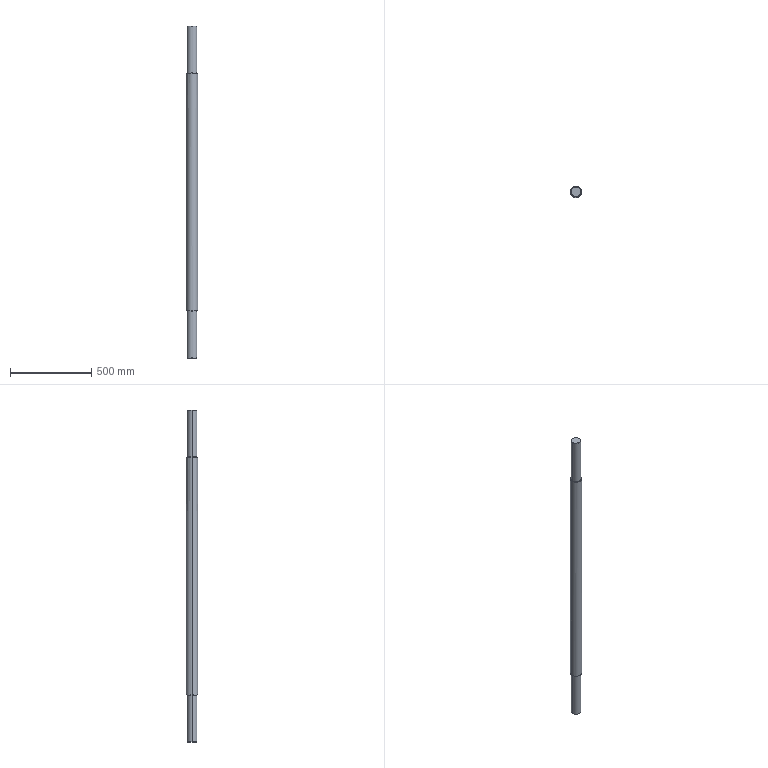Part | STEP file | 1 solid | 34 faces | box 70 x 70 x 2043 mm | volume 7248724 mm3 | cylinder 12 | plane 10 | cone 8 | spline 4 | commonest cylinder face diameters 18 x6 60 x4 70 x2